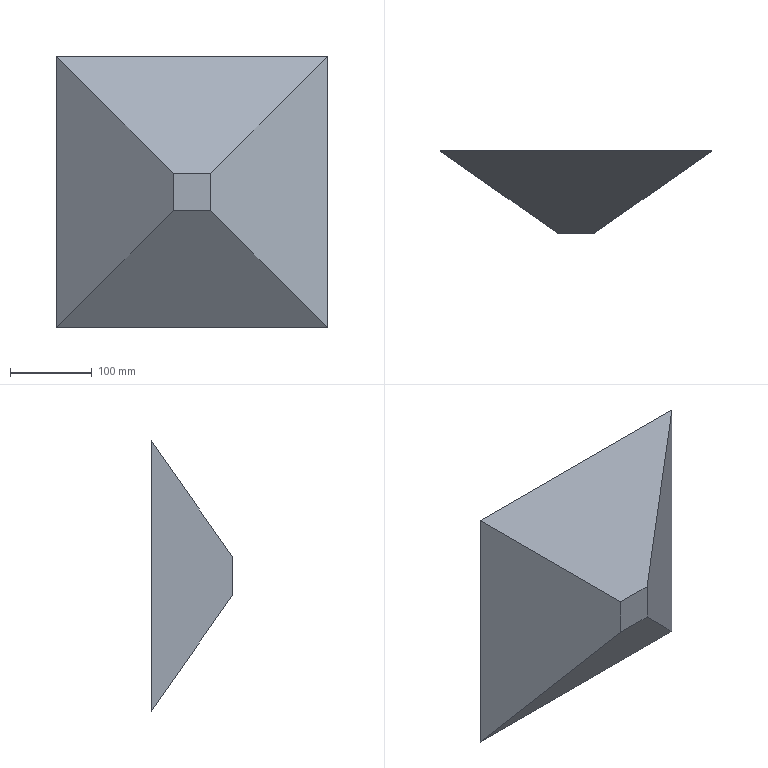Part | SolidWorks | features Blend 1 | 1 solid | 6 faces | box 331.13 x 100 x 331.13 mm | volume 4226115 mm3 | plane 6
STEP:
#1=CARTESIAN_POINT('',(22.75,0.,22.75));
#2=VERTEX_POINT('',#1);
#3=CARTESIAN_POINT('',(22.75,0.,-22.75));
#4=VERTEX_POINT('',#3);
#5=CARTESIAN_POINT('',(22.75,0.,-22.75));
#6=DIRECTION('',(0.,0.,-1.));
#7=VECTOR('',#6,1000.);
#8=LINE('',#5,#7);
#9=EDGE_CURVE('',#2,#4,#8,.T.);
#10=ORIENTED_EDGE('',*,*,#9,.F.);
#11=CARTESIAN_POINT('',(-22.75,0.,22.75));
#12=VERTEX_POINT('',#11);
#13=CARTESIAN_POINT('',(-22.75,0.,22.75));
#14=DIRECTION('',(1.,0.,0.));
#15=VECTOR('',#14,1000.);
#16=LINE('',#13,#15);
#17=EDGE_CURVE('',#12,#2,#16,.T.);
#18=ORIENTED_EDGE('',*,*,#17,.F.);
#19=CARTESIAN_POINT('',(-22.75,0.,-22.75));
#20=VERTEX_POINT('',#19);
#21=CARTESIAN_POINT('',(-22.75,0.,-22.75));
#22=DIRECTION('',(0.,0.,1.));
#23=VECTOR('',#22,1000.);
#24=LINE('',#21,#23);
#25=EDGE_CURVE('',#20,#12,#24,.T.);
#26=ORIENTED_EDGE('',*,*,#25,.F.);
#27=CARTESIAN_POINT('',(-22.75,0.,-22.75));
#28=DIRECTION('',(-1.,0.,0.));
#29=VECTOR('',#28,1000.);
#30=LINE('',#27,#29);
#31=EDGE_CURVE('',#4,#20,#30,.T.);
#32=ORIENTED_EDGE('',*,*,#31,.F.);
#33=EDGE_LOOP('',(#10,#18,#26,#32));
#34=FACE_OUTER_BOUND('',#33,.T.);
#35=CARTESIAN_POINT('',(0.,0.,0.));
#36=DIRECTION('',(0.,1.,0.));
#37=DIRECTION('',(0.,0.,1.));
#38=AXIS2_PLACEMENT_3D('',#35,#36,#37);
#39=PLANE('',#38);
#40=ADVANCED_FACE('',(#34),#39,.F.);
#41=CARTESIAN_POINT('',(165.565,100.,-165.565));
#42=VERTEX_POINT('',#41);
#43=CARTESIAN_POINT('',(165.565,100.,165.565));
#44=VERTEX_POINT('',#43);
#45=CARTESIAN_POINT('',(165.565,100.,165.565));
#46=DIRECTION('',(0.,0.,1.));
#47=VECTOR('',#46,1000.);
#48=LINE('',#45,#47);
#49=EDGE_CURVE('',#42,#44,#48,.T.);
#50=ORIENTED_EDGE('',*,*,#49,.F.);
#51=CARTESIAN_POINT('',(-165.565,100.,-165.565));
#52=VERTEX_POINT('',#51);
#53=CARTESIAN_POINT('',(-165.565,100.,-165.565));
#54=DIRECTION('',(1.,0.,0.));
#55=VECTOR('',#54,1000.);
#56=LINE('',#53,#55);
#57=EDGE_CURVE('',#52,#42,#56,.T.);
#58=ORIENTED_EDGE('',*,*,#57,.F.);
#59=CARTESIAN_POINT('',(-165.565,100.,165.565));
#60=VERTEX_POINT('',#59);
#61=CARTESIAN_POINT('',(-165.565,100.,165.565));
#62=DIRECTION('',(0.,0.,-1.));
#63=VECTOR('',#62,1000.);
#64=LINE('',#61,#63);
#65=EDGE_CURVE('',#60,#52,#64,.T.);
#66=ORIENTED_EDGE('',*,*,#65,.F.);
#67=CARTESIAN_POINT('',(-165.565,100.,165.565));
#68=DIRECTION('',(-1.,0.,0.));
#69=VECTOR('',#68,1000.);
#70=LINE('',#67,#69);
#71=EDGE_CURVE('',#44,#60,#70,.T.);
#72=ORIENTED_EDGE('',*,*,#71,.F.);
#73=EDGE_LOOP('',(#50,#58,#66,#72));
#74=FACE_OUTER_BOUND('',#73,.T.);
#75=CARTESIAN_POINT('',(0.,100.,0.));
#76=DIRECTION('',(0.,-1.,0.));
#77=DIRECTION('',(0.,0.,-1.));
#78=AXIS2_PLACEMENT_3D('',#75,#76,#77);
#79=PLANE('',#78);
#80=ADVANCED_FACE('',(#74),#79,.F.);
#81=CARTESIAN_POINT('',(-165.565,100.,165.565));
#82=DIRECTION('',(0.6337,-0.4437,-0.6337));
#83=VECTOR('',#82,1000.);
#84=LINE('',#81,#83);
#85=EDGE_CURVE('',#60,#12,#84,.T.);
#86=ORIENTED_EDGE('',*,*,#85,.T.);
#87=ORIENTED_EDGE('',*,*,#17,.T.);
#88=CARTESIAN_POINT('',(165.565,100.,165.565));
#89=DIRECTION('',(-0.6337,-0.4437,-0.6337));
#90=VECTOR('',#89,1000.);
#91=LINE('',#88,#90);
#92=EDGE_CURVE('',#44,#2,#91,.T.);
#93=ORIENTED_EDGE('',*,*,#92,.F.);
#94=ORIENTED_EDGE('',*,*,#71,.T.);
#95=EDGE_LOOP('',(#86,#87,#93,#94));
#96=FACE_OUTER_BOUND('',#95,.T.);
#97=CARTESIAN_POINT('',(0.,-10.689,7.485));
#98=DIRECTION('',(0.,0.8192,-0.5736));
#99=DIRECTION('',(0.,0.5736,0.8192));
#100=AXIS2_PLACEMENT_3D('',#97,#98,#99);
#101=PLANE('',#100);
#102=ADVANCED_FACE('',(#96),#101,.F.);
#103=ORIENTED_EDGE('',*,*,#92,.T.);
#104=ORIENTED_EDGE('',*,*,#9,.T.);
#105=CARTESIAN_POINT('',(165.565,100.,-165.565));
#106=DIRECTION('',(-0.6337,-0.4437,0.6337));
#107=VECTOR('',#106,1000.);
#108=LINE('',#105,#107);
#109=EDGE_CURVE('',#42,#4,#108,.T.);
#110=ORIENTED_EDGE('',*,*,#109,.F.);
#111=ORIENTED_EDGE('',*,*,#49,.T.);
#112=EDGE_LOOP('',(#103,#104,#110,#111));
#113=FACE_OUTER_BOUND('',#112,.T.);
#114=CARTESIAN_POINT('',(7.485,-10.689,0.));
#115=DIRECTION('',(-0.5736,0.8192,0.));
#116=DIRECTION('',(-0.8192,-0.5736,0.));
#117=AXIS2_PLACEMENT_3D('',#114,#115,#116);
#118=PLANE('',#117);
#119=ADVANCED_FACE('',(#113),#118,.F.);
#120=CARTESIAN_POINT('',(-165.565,100.,-165.565));
#121=DIRECTION('',(0.6337,-0.4437,0.6337));
#122=VECTOR('',#121,1000.);
#123=LINE('',#120,#122);
#124=EDGE_CURVE('',#52,#20,#123,.T.);
#125=ORIENTED_EDGE('',*,*,#124,.T.);
#126=ORIENTED_EDGE('',*,*,#25,.T.);
#127=ORIENTED_EDGE('',*,*,#85,.F.);
#128=ORIENTED_EDGE('',*,*,#65,.T.);
#129=EDGE_LOOP('',(#125,#126,#127,#128));
#130=FACE_OUTER_BOUND('',#129,.T.);
#131=CARTESIAN_POINT('',(-7.485,-10.689,0.));
#132=DIRECTION('',(0.5736,0.8192,0.));
#133=DIRECTION('',(-0.8192,0.5736,0.));
#134=AXIS2_PLACEMENT_3D('',#131,#132,#133);
#135=PLANE('',#134);
#136=ADVANCED_FACE('',(#130),#135,.F.);
#137=ORIENTED_EDGE('',*,*,#109,.T.);
#138=ORIENTED_EDGE('',*,*,#31,.T.);
#139=ORIENTED_EDGE('',*,*,#124,.F.);
#140=ORIENTED_EDGE('',*,*,#57,.T.);
#141=EDGE_LOOP('',(#137,#138,#139,#140));
#142=FACE_OUTER_BOUND('',#141,.T.);
#143=CARTESIAN_POINT('',(0.,-10.689,-7.485));
#144=DIRECTION('',(0.,0.8192,0.5736));
#145=DIRECTION('',(0.,-0.5736,0.8192));
#146=AXIS2_PLACEMENT_3D('',#143,#144,#145);
#147=PLANE('',#146);
#148=ADVANCED_FACE('',(#142),#147,.F.);
#149=CLOSED_SHELL('',(#40,#80,#102,#119,#136,#148));
#150=MANIFOLD_SOLID_BREP('',#149);
#151=CARTESIAN_POINT('',(0.,0.,0.));
#152=DIRECTION('',(0.,0.,1.));
#153=DIRECTION('',(1.,0.,0.));
#154=AXIS2_PLACEMENT_3D('',#151,#152,#153);
#155=(LENGTH_UNIT()NAMED_UNIT(*)SI_UNIT(.MILLI.,.METRE.));
#156=UNCERTAINTY_MEASURE_WITH_UNIT(LENGTH_MEASURE(0.00001),#155,'','');
#157=(NAMED_UNIT(*)PLANE_ANGLE_UNIT()SI_UNIT($,.RADIAN.));
#158=(NAMED_UNIT(*)SI_UNIT($,.STERADIAN.)SOLID_ANGLE_UNIT());
#159=(GEOMETRIC_REPRESENTATION_CONTEXT(3)GLOBAL_UNCERTAINTY_ASSIGNED_CONTEXT((#156))GLOBAL_UNIT_ASSIGNED_CONTEXT((#155,#157,#158))REPRESENTATION_CONTEXT('',''));
#160=ADVANCED_BREP_SHAPE_REPRESENTATION('',(#150,#154),#159);